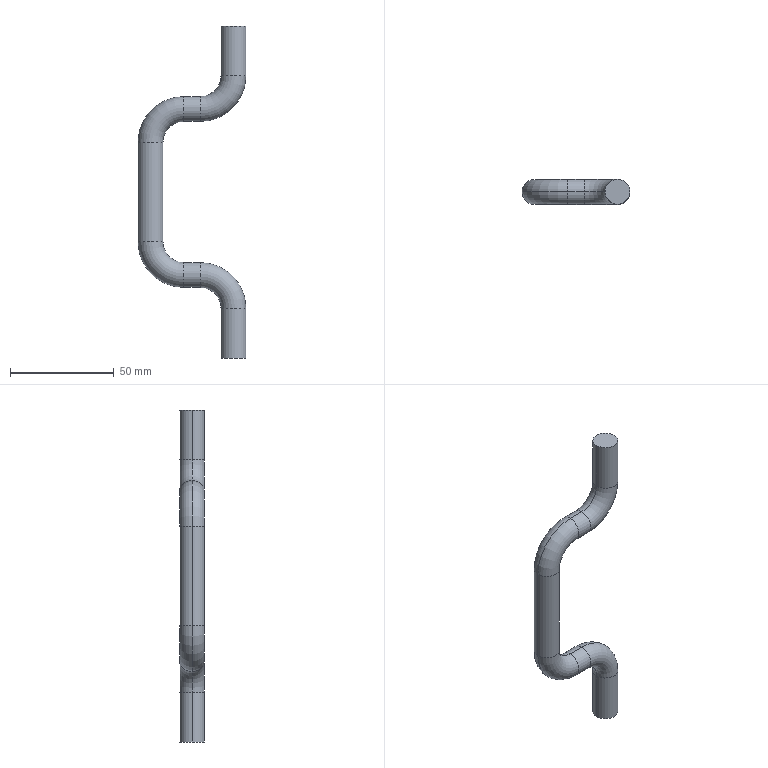Part | SolidWorks | features Sweep 1 | 1 solid | 20 faces | box 52 x 12 x 160 mm | volume 24037 mm3 | cylinder 10 | torus 8 | plane 2 | commonest cylinder face diameters 12 x10
STEP:
#1=CARTESIAN_POINT('',(6.,0.,-24.));
#2=VERTEX_POINT('',#1);
#3=CARTESIAN_POINT('',(-6.,0.,-24.));
#4=VERTEX_POINT('',#3);
#5=CARTESIAN_POINT('',(0.,0.,-24.));
#6=DIRECTION('',(0.,0.,1.));
#7=DIRECTION('',(1.,0.,0.));
#8=AXIS2_PLACEMENT_3D('',#5,#6,#7);
#9=CIRCLE('',#8,6.);
#10=EDGE_CURVE('',#2,#4,#9,.T.);
#11=ORIENTED_EDGE('',*,*,#10,.F.);
#12=CARTESIAN_POINT('',(-16.,0.,-46.));
#13=VERTEX_POINT('',#12);
#14=CARTESIAN_POINT('',(-16.,0.,-24.));
#15=DIRECTION('',(0.,1.,0.));
#16=DIRECTION('',(0.,0.,1.));
#17=AXIS2_PLACEMENT_3D('',#14,#15,#16);
#18=CIRCLE('',#17,22.);
#19=EDGE_CURVE('',#2,#13,#18,.T.);
#20=ORIENTED_EDGE('',*,*,#19,.T.);
#21=CARTESIAN_POINT('',(-16.,0.,-34.));
#22=VERTEX_POINT('',#21);
#23=CARTESIAN_POINT('',(-16.,0.,-40.));
#24=DIRECTION('',(1.,0.,0.));
#25=DIRECTION('',(0.,0.,-1.));
#26=AXIS2_PLACEMENT_3D('',#23,#24,#25);
#27=CIRCLE('',#26,6.);
#28=EDGE_CURVE('',#13,#22,#27,.T.);
#29=ORIENTED_EDGE('',*,*,#28,.T.);
#30=CARTESIAN_POINT('',(-16.,0.,-24.));
#31=DIRECTION('',(0.,1.,0.));
#32=DIRECTION('',(0.,0.,1.));
#33=AXIS2_PLACEMENT_3D('',#30,#31,#32);
#34=CIRCLE('',#33,10.);
#35=EDGE_CURVE('',#4,#22,#34,.T.);
#36=ORIENTED_EDGE('',*,*,#35,.F.);
#37=EDGE_LOOP('',(#11,#20,#29,#36));
#38=FACE_OUTER_BOUND('',#37,.T.);
#39=CARTESIAN_POINT('',(-16.,0.,-24.));
#40=DIRECTION('',(0.,1.,0.));
#41=DIRECTION('',(0.,0.,1.));
#42=AXIS2_PLACEMENT_3D('',#39,#40,#41);
#43=TOROIDAL_SURFACE('',#42,16.,6.);
#44=ADVANCED_FACE('',(#38),#43,.T.);
#45=CARTESIAN_POINT('',(-24.,0.,-34.));
#46=VERTEX_POINT('',#45);
#47=CARTESIAN_POINT('',(-24.,0.,-46.));
#48=VERTEX_POINT('',#47);
#49=CARTESIAN_POINT('',(-24.,0.,-40.));
#50=DIRECTION('',(1.,0.,0.));
#51=DIRECTION('',(0.,0.,-1.));
#52=AXIS2_PLACEMENT_3D('',#49,#50,#51);
#53=CIRCLE('',#52,6.);
#54=EDGE_CURVE('',#46,#48,#53,.T.);
#55=ORIENTED_EDGE('',*,*,#54,.F.);
#56=CARTESIAN_POINT('',(-46.,0.,-56.));
#57=VERTEX_POINT('',#56);
#58=CARTESIAN_POINT('',(-24.,0.,-56.));
#59=DIRECTION('',(0.,-1.,0.));
#60=DIRECTION('',(0.,0.,-1.));
#61=AXIS2_PLACEMENT_3D('',#58,#59,#60);
#62=CIRCLE('',#61,22.);
#63=EDGE_CURVE('',#46,#57,#62,.T.);
#64=ORIENTED_EDGE('',*,*,#63,.T.);
#65=CARTESIAN_POINT('',(-34.,0.,-56.));
#66=VERTEX_POINT('',#65);
#67=CARTESIAN_POINT('',(-40.,0.,-56.));
#68=DIRECTION('',(0.,0.,1.));
#69=DIRECTION('',(1.,0.,0.));
#70=AXIS2_PLACEMENT_3D('',#67,#68,#69);
#71=CIRCLE('',#70,6.);
#72=EDGE_CURVE('',#57,#66,#71,.T.);
#73=ORIENTED_EDGE('',*,*,#72,.T.);
#74=CARTESIAN_POINT('',(-24.,0.,-56.));
#75=DIRECTION('',(0.,-1.,0.));
#76=DIRECTION('',(0.,0.,-1.));
#77=AXIS2_PLACEMENT_3D('',#74,#75,#76);
#78=CIRCLE('',#77,10.);
#79=EDGE_CURVE('',#48,#66,#78,.T.);
#80=ORIENTED_EDGE('',*,*,#79,.F.);
#81=EDGE_LOOP('',(#55,#64,#73,#80));
#82=FACE_OUTER_BOUND('',#81,.T.);
#83=CARTESIAN_POINT('',(-24.,0.,-56.));
#84=DIRECTION('',(0.,-1.,0.));
#85=DIRECTION('',(0.,0.,-1.));
#86=AXIS2_PLACEMENT_3D('',#83,#84,#85);
#87=TOROIDAL_SURFACE('',#86,16.,6.);
#88=ADVANCED_FACE('',(#82),#87,.T.);
#89=CARTESIAN_POINT('',(-46.,0.,-104.));
#90=VERTEX_POINT('',#89);
#91=CARTESIAN_POINT('',(-34.,0.,-104.));
#92=VERTEX_POINT('',#91);
#93=CARTESIAN_POINT('',(-40.,0.,-104.));
#94=DIRECTION('',(0.,0.,1.));
#95=DIRECTION('',(1.,0.,0.));
#96=AXIS2_PLACEMENT_3D('',#93,#94,#95);
#97=CIRCLE('',#96,6.);
#98=EDGE_CURVE('',#90,#92,#97,.T.);
#99=ORIENTED_EDGE('',*,*,#98,.F.);
#100=CARTESIAN_POINT('',(-24.,0.,-126.));
#101=VERTEX_POINT('',#100);
#102=CARTESIAN_POINT('',(-24.,0.,-104.));
#103=DIRECTION('',(0.,-1.,0.));
#104=DIRECTION('',(0.,0.,-1.));
#105=AXIS2_PLACEMENT_3D('',#102,#103,#104);
#106=CIRCLE('',#105,22.);
#107=EDGE_CURVE('',#90,#101,#106,.T.);
#108=ORIENTED_EDGE('',*,*,#107,.T.);
#109=CARTESIAN_POINT('',(-24.,0.,-114.));
#110=VERTEX_POINT('',#109);
#111=CARTESIAN_POINT('',(-24.,0.,-120.));
#112=DIRECTION('',(-1.,0.,0.));
#113=DIRECTION('',(0.,0.,1.));
#114=AXIS2_PLACEMENT_3D('',#111,#112,#113);
#115=CIRCLE('',#114,6.);
#116=EDGE_CURVE('',#101,#110,#115,.T.);
#117=ORIENTED_EDGE('',*,*,#116,.T.);
#118=CARTESIAN_POINT('',(-24.,0.,-104.));
#119=DIRECTION('',(0.,-1.,0.));
#120=DIRECTION('',(0.,0.,-1.));
#121=AXIS2_PLACEMENT_3D('',#118,#119,#120);
#122=CIRCLE('',#121,10.);
#123=EDGE_CURVE('',#92,#110,#122,.T.);
#124=ORIENTED_EDGE('',*,*,#123,.F.);
#125=EDGE_LOOP('',(#99,#108,#117,#124));
#126=FACE_OUTER_BOUND('',#125,.T.);
#127=CARTESIAN_POINT('',(-24.,0.,-104.));
#128=DIRECTION('',(0.,-1.,0.));
#129=DIRECTION('',(0.,0.,-1.));
#130=AXIS2_PLACEMENT_3D('',#127,#128,#129);
#131=TOROIDAL_SURFACE('',#130,16.,6.);
#132=ADVANCED_FACE('',(#126),#131,.T.);
#133=CARTESIAN_POINT('',(-16.,0.,-114.));
#134=VERTEX_POINT('',#133);
#135=CARTESIAN_POINT('',(-16.,0.,-126.));
#136=VERTEX_POINT('',#135);
#137=CARTESIAN_POINT('',(-16.,0.,-120.));
#138=DIRECTION('',(-1.,0.,0.));
#139=DIRECTION('',(0.,0.,1.));
#140=AXIS2_PLACEMENT_3D('',#137,#138,#139);
#141=CIRCLE('',#140,6.);
#142=EDGE_CURVE('',#134,#136,#141,.T.);
#143=ORIENTED_EDGE('',*,*,#142,.F.);
#144=CARTESIAN_POINT('',(6.,0.,-136.));
#145=VERTEX_POINT('',#144);
#146=CARTESIAN_POINT('',(-16.,0.,-136.));
#147=DIRECTION('',(0.,1.,0.));
#148=DIRECTION('',(0.,0.,1.));
#149=AXIS2_PLACEMENT_3D('',#146,#147,#148);
#150=CIRCLE('',#149,22.);
#151=EDGE_CURVE('',#134,#145,#150,.T.);
#152=ORIENTED_EDGE('',*,*,#151,.T.);
#153=CARTESIAN_POINT('',(-6.,0.,-136.));
#154=VERTEX_POINT('',#153);
#155=CARTESIAN_POINT('',(0.,0.,-136.));
#156=DIRECTION('',(0.,0.,1.));
#157=DIRECTION('',(1.,0.,0.));
#158=AXIS2_PLACEMENT_3D('',#155,#156,#157);
#159=CIRCLE('',#158,6.);
#160=EDGE_CURVE('',#145,#154,#159,.T.);
#161=ORIENTED_EDGE('',*,*,#160,.T.);
#162=CARTESIAN_POINT('',(-16.,0.,-136.));
#163=DIRECTION('',(0.,1.,0.));
#164=DIRECTION('',(0.,0.,1.));
#165=AXIS2_PLACEMENT_3D('',#162,#163,#164);
#166=CIRCLE('',#165,10.);
#167=EDGE_CURVE('',#136,#154,#166,.T.);
#168=ORIENTED_EDGE('',*,*,#167,.F.);
#169=EDGE_LOOP('',(#143,#152,#161,#168));
#170=FACE_OUTER_BOUND('',#169,.T.);
#171=CARTESIAN_POINT('',(-16.,0.,-136.));
#172=DIRECTION('',(0.,1.,0.));
#173=DIRECTION('',(0.,0.,1.));
#174=AXIS2_PLACEMENT_3D('',#171,#172,#173);
#175=TOROIDAL_SURFACE('',#174,16.,6.);
#176=ADVANCED_FACE('',(#170),#175,.T.);
#177=ORIENTED_EDGE('',*,*,#10,.T.);
#178=CARTESIAN_POINT('',(-6.,0.,0.));
#179=VERTEX_POINT('',#178);
#180=CARTESIAN_POINT('',(-6.,0.,-24.));
#181=DIRECTION('',(0.,0.,1.));
#182=VECTOR('',#181,1000.);
#183=LINE('',#180,#182);
#184=EDGE_CURVE('',#4,#179,#183,.T.);
#185=ORIENTED_EDGE('',*,*,#184,.T.);
#186=CARTESIAN_POINT('',(6.,0.,0.));
#187=VERTEX_POINT('',#186);
#188=CARTESIAN_POINT('',(0.,0.,0.));
#189=DIRECTION('',(0.,0.,1.));
#190=DIRECTION('',(1.,0.,0.));
#191=AXIS2_PLACEMENT_3D('',#188,#189,#190);
#192=CIRCLE('',#191,6.);
#193=EDGE_CURVE('',#187,#179,#192,.T.);
#194=ORIENTED_EDGE('',*,*,#193,.F.);
#195=CARTESIAN_POINT('',(6.,0.,-24.));
#196=DIRECTION('',(0.,0.,1.));
#197=VECTOR('',#196,1000.);
#198=LINE('',#195,#197);
#199=EDGE_CURVE('',#2,#187,#198,.T.);
#200=ORIENTED_EDGE('',*,*,#199,.F.);
#201=EDGE_LOOP('',(#177,#185,#194,#200));
#202=FACE_OUTER_BOUND('',#201,.T.);
#203=CARTESIAN_POINT('',(0.,0.,-24.));
#204=DIRECTION('',(0.,0.,1.));
#205=DIRECTION('',(1.,0.,0.));
#206=AXIS2_PLACEMENT_3D('',#203,#204,#205);
#207=CYLINDRICAL_SURFACE('',#206,6.);
#208=ADVANCED_FACE('',(#202),#207,.T.);
#209=ORIENTED_EDGE('',*,*,#28,.F.);
#210=CARTESIAN_POINT('',(-16.,0.,-46.));
#211=DIRECTION('',(-1.,0.,0.));
#212=VECTOR('',#211,1000.);
#213=LINE('',#210,#212);
#214=EDGE_CURVE('',#13,#48,#213,.T.);
#215=ORIENTED_EDGE('',*,*,#214,.T.);
#216=CARTESIAN_POINT('',(-24.,0.,-40.));
#217=DIRECTION('',(1.,0.,0.));
#218=DIRECTION('',(0.,0.,-1.));
#219=AXIS2_PLACEMENT_3D('',#216,#217,#218);
#220=CIRCLE('',#219,6.);
#221=EDGE_CURVE('',#48,#46,#220,.T.);
#222=ORIENTED_EDGE('',*,*,#221,.T.);
#223=CARTESIAN_POINT('',(-16.,0.,-34.));
#224=DIRECTION('',(-1.,0.,0.));
#225=VECTOR('',#224,1000.);
#226=LINE('',#223,#225);
#227=EDGE_CURVE('',#22,#46,#226,.T.);
#228=ORIENTED_EDGE('',*,*,#227,.F.);
#229=EDGE_LOOP('',(#209,#215,#222,#228));
#230=FACE_OUTER_BOUND('',#229,.T.);
#231=CARTESIAN_POINT('',(-16.,0.,-40.));
#232=DIRECTION('',(-1.,0.,0.));
#233=DIRECTION('',(0.,0.,1.));
#234=AXIS2_PLACEMENT_3D('',#231,#232,#233);
#235=CYLINDRICAL_SURFACE('',#234,6.);
#236=ADVANCED_FACE('',(#230),#235,.T.);
#237=CARTESIAN_POINT('',(-40.,0.,-56.));
#238=DIRECTION('',(0.,0.,1.));
#239=DIRECTION('',(1.,0.,0.));
#240=AXIS2_PLACEMENT_3D('',#237,#238,#239);
#241=CIRCLE('',#240,6.);
#242=EDGE_CURVE('',#66,#57,#241,.T.);
#243=ORIENTED_EDGE('',*,*,#242,.F.);
#244=CARTESIAN_POINT('',(-34.,0.,-56.));
#245=DIRECTION('',(0.,0.,-1.));
#246=VECTOR('',#245,1000.);
#247=LINE('',#244,#246);
#248=EDGE_CURVE('',#66,#92,#247,.T.);
#249=ORIENTED_EDGE('',*,*,#248,.T.);
#250=CARTESIAN_POINT('',(-40.,0.,-104.));
#251=DIRECTION('',(0.,0.,1.));
#252=DIRECTION('',(1.,0.,0.));
#253=AXIS2_PLACEMENT_3D('',#250,#251,#252);
#254=CIRCLE('',#253,6.);
#255=EDGE_CURVE('',#92,#90,#254,.T.);
#256=ORIENTED_EDGE('',*,*,#255,.T.);
#257=CARTESIAN_POINT('',(-46.,0.,-56.));
#258=DIRECTION('',(0.,0.,-1.));
#259=VECTOR('',#258,1000.);
#260=LINE('',#257,#259);
#261=EDGE_CURVE('',#57,#90,#260,.T.);
#262=ORIENTED_EDGE('',*,*,#261,.F.);
#263=EDGE_LOOP('',(#243,#249,#256,#262));
#264=FACE_OUTER_BOUND('',#263,.T.);
#265=CARTESIAN_POINT('',(-40.,0.,-56.));
#266=DIRECTION('',(0.,0.,-1.));
#267=DIRECTION('',(-1.,0.,0.));
#268=AXIS2_PLACEMENT_3D('',#265,#266,#267);
#269=CYLINDRICAL_SURFACE('',#268,6.);
#270=ADVANCED_FACE('',(#264),#269,.T.);
#271=CARTESIAN_POINT('',(-24.,0.,-120.));
#272=DIRECTION('',(-1.,0.,0.));
#273=DIRECTION('',(0.,0.,1.));
#274=AXIS2_PLACEMENT_3D('',#271,#272,#273);
#275=CIRCLE('',#274,6.);
#276=EDGE_CURVE('',#110,#101,#275,.T.);
#277=ORIENTED_EDGE('',*,*,#276,.F.);
#278=CARTESIAN_POINT('',(-24.,0.,-114.));
#279=DIRECTION('',(1.,0.,0.));
#280=VECTOR('',#279,1000.);
#281=LINE('',#278,#280);
#282=EDGE_CURVE('',#110,#134,#281,.T.);
#283=ORIENTED_EDGE('',*,*,#282,.T.);
#284=ORIENTED_EDGE('',*,*,#142,.T.);
#285=CARTESIAN_POINT('',(-24.,0.,-126.));
#286=DIRECTION('',(1.,0.,0.));
#287=VECTOR('',#286,1000.);
#288=LINE('',#285,#287);
#289=EDGE_CURVE('',#101,#136,#288,.T.);
#290=ORIENTED_EDGE('',*,*,#289,.F.);
#291=EDGE_LOOP('',(#277,#283,#284,#290));
#292=FACE_OUTER_BOUND('',#291,.T.);
#293=CARTESIAN_POINT('',(-24.,0.,-120.));
#294=DIRECTION('',(1.,0.,0.));
#295=DIRECTION('',(0.,0.,-1.));
#296=AXIS2_PLACEMENT_3D('',#293,#294,#295);
#297=CYLINDRICAL_SURFACE('',#296,6.);
#298=ADVANCED_FACE('',(#292),#297,.T.);
#299=ORIENTED_EDGE('',*,*,#160,.F.);
#300=CARTESIAN_POINT('',(6.,0.,-160.));
#301=VERTEX_POINT('',#300);
#302=CARTESIAN_POINT('',(6.,0.,-136.));
#303=DIRECTION('',(0.,0.,-1.));
#304=VECTOR('',#303,1000.);
#305=LINE('',#302,#304);
#306=EDGE_CURVE('',#145,#301,#305,.T.);
#307=ORIENTED_EDGE('',*,*,#306,.T.);
#308=CARTESIAN_POINT('',(-6.,0.,-160.));
#309=VERTEX_POINT('',#308);
#310=CARTESIAN_POINT('',(0.,0.,-160.));
#311=DIRECTION('',(0.,0.,1.));
#312=DIRECTION('',(1.,0.,0.));
#313=AXIS2_PLACEMENT_3D('',#310,#311,#312);
#314=CIRCLE('',#313,6.);
#315=EDGE_CURVE('',#301,#309,#314,.T.);
#316=ORIENTED_EDGE('',*,*,#315,.T.);
#317=CARTESIAN_POINT('',(-6.,0.,-136.));
#318=DIRECTION('',(0.,0.,-1.));
#319=VECTOR('',#318,1000.);
#320=LINE('',#317,#319);
#321=EDGE_CURVE('',#154,#309,#320,.T.);
#322=ORIENTED_EDGE('',*,*,#321,.F.);
#323=EDGE_LOOP('',(#299,#307,#316,#322));
#324=FACE_OUTER_BOUND('',#323,.T.);
#325=CARTESIAN_POINT('',(0.,0.,-136.));
#326=DIRECTION('',(0.,0.,-1.));
#327=DIRECTION('',(-1.,0.,0.));
#328=AXIS2_PLACEMENT_3D('',#325,#326,#327);
#329=CYLINDRICAL_SURFACE('',#328,6.);
#330=ADVANCED_FACE('',(#324),#329,.T.);
#331=ORIENTED_EDGE('',*,*,#306,.F.);
#332=CARTESIAN_POINT('',(0.,0.,-136.));
#333=DIRECTION('',(0.,0.,1.));
#334=DIRECTION('',(1.,0.,0.));
#335=AXIS2_PLACEMENT_3D('',#332,#333,#334);
#336=CIRCLE('',#335,6.);
#337=EDGE_CURVE('',#154,#145,#336,.T.);
#338=ORIENTED_EDGE('',*,*,#337,.F.);
#339=ORIENTED_EDGE('',*,*,#321,.T.);
#340=CARTESIAN_POINT('',(0.,0.,-160.));
#341=DIRECTION('',(0.,0.,1.));
#342=DIRECTION('',(1.,0.,0.));
#343=AXIS2_PLACEMENT_3D('',#340,#341,#342);
#344=CIRCLE('',#343,6.);
#345=EDGE_CURVE('',#309,#301,#344,.T.);
#346=ORIENTED_EDGE('',*,*,#345,.T.);
#347=EDGE_LOOP('',(#331,#338,#339,#346));
#348=FACE_OUTER_BOUND('',#347,.T.);
#349=CARTESIAN_POINT('',(0.,0.,-136.));
#350=DIRECTION('',(0.,0.,-1.));
#351=DIRECTION('',(-1.,0.,0.));
#352=AXIS2_PLACEMENT_3D('',#349,#350,#351);
#353=CYLINDRICAL_SURFACE('',#352,6.);
#354=ADVANCED_FACE('',(#348),#353,.T.);
#355=ORIENTED_EDGE('',*,*,#151,.F.);
#356=CARTESIAN_POINT('',(-16.,0.,-120.));
#357=DIRECTION('',(-1.,0.,0.));
#358=DIRECTION('',(0.,0.,1.));
#359=AXIS2_PLACEMENT_3D('',#356,#357,#358);
#360=CIRCLE('',#359,6.);
#361=EDGE_CURVE('',#136,#134,#360,.T.);
#362=ORIENTED_EDGE('',*,*,#361,.F.);
#363=ORIENTED_EDGE('',*,*,#167,.T.);
#364=ORIENTED_EDGE('',*,*,#337,.T.);
#365=EDGE_LOOP('',(#355,#362,#363,#364));
#366=FACE_OUTER_BOUND('',#365,.T.);
#367=CARTESIAN_POINT('',(-16.,0.,-136.));
#368=DIRECTION('',(0.,1.,0.));
#369=DIRECTION('',(0.,0.,1.));
#370=AXIS2_PLACEMENT_3D('',#367,#368,#369);
#371=TOROIDAL_SURFACE('',#370,16.,6.);
#372=ADVANCED_FACE('',(#366),#371,.T.);
#373=ORIENTED_EDGE('',*,*,#282,.F.);
#374=ORIENTED_EDGE('',*,*,#116,.F.);
#375=ORIENTED_EDGE('',*,*,#289,.T.);
#376=ORIENTED_EDGE('',*,*,#361,.T.);
#377=EDGE_LOOP('',(#373,#374,#375,#376));
#378=FACE_OUTER_BOUND('',#377,.T.);
#379=CARTESIAN_POINT('',(-24.,0.,-120.));
#380=DIRECTION('',(1.,0.,0.));
#381=DIRECTION('',(0.,0.,-1.));
#382=AXIS2_PLACEMENT_3D('',#379,#380,#381);
#383=CYLINDRICAL_SURFACE('',#382,6.);
#384=ADVANCED_FACE('',(#378),#383,.T.);
#385=ORIENTED_EDGE('',*,*,#107,.F.);
#386=ORIENTED_EDGE('',*,*,#255,.F.);
#387=ORIENTED_EDGE('',*,*,#123,.T.);
#388=ORIENTED_EDGE('',*,*,#276,.T.);
#389=EDGE_LOOP('',(#385,#386,#387,#388));
#390=FACE_OUTER_BOUND('',#389,.T.);
#391=CARTESIAN_POINT('',(-24.,0.,-104.));
#392=DIRECTION('',(0.,-1.,0.));
#393=DIRECTION('',(0.,0.,-1.));
#394=AXIS2_PLACEMENT_3D('',#391,#392,#393);
#395=TOROIDAL_SURFACE('',#394,16.,6.);
#396=ADVANCED_FACE('',(#390),#395,.T.);
#397=ORIENTED_EDGE('',*,*,#248,.F.);
#398=ORIENTED_EDGE('',*,*,#72,.F.);
#399=ORIENTED_EDGE('',*,*,#261,.T.);
#400=ORIENTED_EDGE('',*,*,#98,.T.);
#401=EDGE_LOOP('',(#397,#398,#399,#400));
#402=FACE_OUTER_BOUND('',#401,.T.);
#403=CARTESIAN_POINT('',(-40.,0.,-56.));
#404=DIRECTION('',(0.,0.,-1.));
#405=DIRECTION('',(-1.,0.,0.));
#406=AXIS2_PLACEMENT_3D('',#403,#404,#405);
#407=CYLINDRICAL_SURFACE('',#406,6.);
#408=ADVANCED_FACE('',(#402),#407,.T.);
#409=ORIENTED_EDGE('',*,*,#63,.F.);
#410=ORIENTED_EDGE('',*,*,#221,.F.);
#411=ORIENTED_EDGE('',*,*,#79,.T.);
#412=ORIENTED_EDGE('',*,*,#242,.T.);
#413=EDGE_LOOP('',(#409,#410,#411,#412));
#414=FACE_OUTER_BOUND('',#413,.T.);
#415=CARTESIAN_POINT('',(-24.,0.,-56.));
#416=DIRECTION('',(0.,-1.,0.));
#417=DIRECTION('',(0.,0.,-1.));
#418=AXIS2_PLACEMENT_3D('',#415,#416,#417);
#419=TOROIDAL_SURFACE('',#418,16.,6.);
#420=ADVANCED_FACE('',(#414),#419,.T.);
#421=ORIENTED_EDGE('',*,*,#214,.F.);
#422=CARTESIAN_POINT('',(-16.,0.,-40.));
#423=DIRECTION('',(1.,0.,0.));
#424=DIRECTION('',(0.,0.,-1.));
#425=AXIS2_PLACEMENT_3D('',#422,#423,#424);
#426=CIRCLE('',#425,6.);
#427=EDGE_CURVE('',#22,#13,#426,.T.);
#428=ORIENTED_EDGE('',*,*,#427,.F.);
#429=ORIENTED_EDGE('',*,*,#227,.T.);
#430=ORIENTED_EDGE('',*,*,#54,.T.);
#431=EDGE_LOOP('',(#421,#428,#429,#430));
#432=FACE_OUTER_BOUND('',#431,.T.);
#433=CARTESIAN_POINT('',(-16.,0.,-40.));
#434=DIRECTION('',(-1.,0.,0.));
#435=DIRECTION('',(0.,0.,1.));
#436=AXIS2_PLACEMENT_3D('',#433,#434,#435);
#437=CYLINDRICAL_SURFACE('',#436,6.);
#438=ADVANCED_FACE('',(#432),#437,.T.);
#439=ORIENTED_EDGE('',*,*,#19,.F.);
#440=CARTESIAN_POINT('',(0.,0.,-24.));
#441=DIRECTION('',(0.,0.,1.));
#442=DIRECTION('',(1.,0.,0.));
#443=AXIS2_PLACEMENT_3D('',#440,#441,#442);
#444=CIRCLE('',#443,6.);
#445=EDGE_CURVE('',#4,#2,#444,.T.);
#446=ORIENTED_EDGE('',*,*,#445,.F.);
#447=ORIENTED_EDGE('',*,*,#35,.T.);
#448=ORIENTED_EDGE('',*,*,#427,.T.);
#449=EDGE_LOOP('',(#439,#446,#447,#448));
#450=FACE_OUTER_BOUND('',#449,.T.);
#451=CARTESIAN_POINT('',(-16.,0.,-24.));
#452=DIRECTION('',(0.,1.,0.));
#453=DIRECTION('',(0.,0.,1.));
#454=AXIS2_PLACEMENT_3D('',#451,#452,#453);
#455=TOROIDAL_SURFACE('',#454,16.,6.);
#456=ADVANCED_FACE('',(#450),#455,.T.);
#457=ORIENTED_EDGE('',*,*,#184,.F.);
#458=ORIENTED_EDGE('',*,*,#445,.T.);
#459=ORIENTED_EDGE('',*,*,#199,.T.);
#460=CARTESIAN_POINT('',(0.,0.,0.));
#461=DIRECTION('',(0.,0.,1.));
#462=DIRECTION('',(1.,0.,0.));
#463=AXIS2_PLACEMENT_3D('',#460,#461,#462);
#464=CIRCLE('',#463,6.);
#465=EDGE_CURVE('',#179,#187,#464,.T.);
#466=ORIENTED_EDGE('',*,*,#465,.F.);
#467=EDGE_LOOP('',(#457,#458,#459,#466));
#468=FACE_OUTER_BOUND('',#467,.T.);
#469=CARTESIAN_POINT('',(0.,0.,-24.));
#470=DIRECTION('',(0.,0.,1.));
#471=DIRECTION('',(1.,0.,0.));
#472=AXIS2_PLACEMENT_3D('',#469,#470,#471);
#473=CYLINDRICAL_SURFACE('',#472,6.);
#474=ADVANCED_FACE('',(#468),#473,.T.);
#475=ORIENTED_EDGE('',*,*,#345,.F.);
#476=ORIENTED_EDGE('',*,*,#315,.F.);
#477=EDGE_LOOP('',(#475,#476));
#478=FACE_OUTER_BOUND('',#477,.T.);
#479=CARTESIAN_POINT('',(0.,0.,-160.));
#480=DIRECTION('',(0.,0.,1.));
#481=DIRECTION('',(1.,0.,0.));
#482=AXIS2_PLACEMENT_3D('',#479,#480,#481);
#483=PLANE('',#482);
#484=ADVANCED_FACE('',(#478),#483,.F.);
#485=ORIENTED_EDGE('',*,*,#193,.T.);
#486=ORIENTED_EDGE('',*,*,#465,.T.);
#487=EDGE_LOOP('',(#485,#486));
#488=FACE_OUTER_BOUND('',#487,.T.);
#489=CARTESIAN_POINT('',(0.,0.,0.));
#490=DIRECTION('',(0.,0.,1.));
#491=DIRECTION('',(1.,0.,0.));
#492=AXIS2_PLACEMENT_3D('',#489,#490,#491);
#493=PLANE('',#492);
#494=ADVANCED_FACE('',(#488),#493,.T.);
#495=CLOSED_SHELL('',(#44,#88,#132,#176,#208,#236,#270,#298,#330,#354,#372,#384,#396,#408,#420,#438,#456,#474,#484,#494));
#496=MANIFOLD_SOLID_BREP('',#495);
#497=CARTESIAN_POINT('',(0.,0.,0.));
#498=DIRECTION('',(0.,0.,1.));
#499=DIRECTION('',(1.,0.,0.));
#500=AXIS2_PLACEMENT_3D('',#497,#498,#499);
#501=(LENGTH_UNIT()NAMED_UNIT(*)SI_UNIT(.MILLI.,.METRE.));
#502=UNCERTAINTY_MEASURE_WITH_UNIT(LENGTH_MEASURE(0.00001),#501,'','');
#503=(NAMED_UNIT(*)PLANE_ANGLE_UNIT()SI_UNIT($,.RADIAN.));
#504=(NAMED_UNIT(*)SI_UNIT($,.STERADIAN.)SOLID_ANGLE_UNIT());
#505=(GEOMETRIC_REPRESENTATION_CONTEXT(3)GLOBAL_UNCERTAINTY_ASSIGNED_CONTEXT((#502))GLOBAL_UNIT_ASSIGNED_CONTEXT((#501,#503,#504))REPRESENTATION_CONTEXT('',''));
#506=ADVANCED_BREP_SHAPE_REPRESENTATION('',(#496,#500),#505);